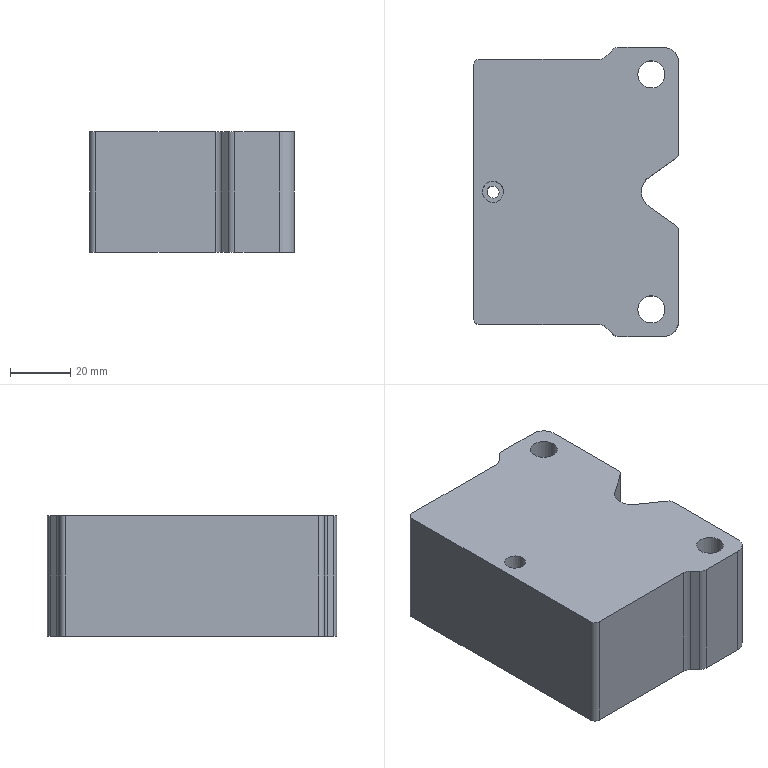Part | NX | features PS-41 2 | 1 solid | 33 faces | box 68 x 96 x 40 mm | volume 229796 mm3 | cylinder 17 | plane 16 | commonest cylinder face diameters 4 x4 6 x4 9 x2 10 x2 14.5 x2 4.001 x1
STEP:
#1=CARTESIAN_POINT('',(4197.993,-814.122,900.716));
#2=VERTEX_POINT('',#1);
#3=CARTESIAN_POINT('',(4158.236,-814.122,900.716));
#4=VERTEX_POINT('',#3);
#5=CARTESIAN_POINT('',(4222.236,-814.122,900.716));
#6=DIRECTION('',(-1.,0.,0.));
#7=VECTOR('',#6,1000.);
#8=LINE('',#5,#7);
#9=EDGE_CURVE('',#2,#4,#8,.T.);
#10=ORIENTED_EDGE('',*,*,#9,.F.);
#11=CARTESIAN_POINT('',(4197.993,-814.122,860.716));
#12=VERTEX_POINT('',#11);
#13=CARTESIAN_POINT('',(4197.993,-814.122,860.716));
#14=DIRECTION('',(0.,0.,-1.));
#15=VECTOR('',#14,1000.);
#16=LINE('',#13,#15);
#17=EDGE_CURVE('',#2,#12,#16,.T.);
#18=ORIENTED_EDGE('',*,*,#17,.T.);
#19=CARTESIAN_POINT('',(4158.236,-814.122,860.716));
#20=VERTEX_POINT('',#19);
#21=CARTESIAN_POINT('',(4222.236,-814.122,860.716));
#22=DIRECTION('',(-1.,0.,0.));
#23=VECTOR('',#22,1000.);
#24=LINE('',#21,#23);
#25=EDGE_CURVE('',#12,#20,#24,.T.);
#26=ORIENTED_EDGE('',*,*,#25,.T.);
#27=CARTESIAN_POINT('',(4158.236,-814.122,860.716));
#28=DIRECTION('',(0.,0.,-1.));
#29=VECTOR('',#28,1000.);
#30=LINE('',#27,#29);
#31=EDGE_CURVE('',#20,#4,#30,.F.);
#32=ORIENTED_EDGE('',*,*,#31,.T.);
#33=EDGE_LOOP('',(#10,#18,#26,#32));
#34=FACE_BOUND('',#33,.T.);
#35=CARTESIAN_POINT('',(4201.082,-814.122,860.716));
#36=DIRECTION('',(0.,1.,0.));
#37=DIRECTION('',(0.,0.,1.));
#38=AXIS2_PLACEMENT_3D('',#35,#36,#37);
#39=PLANE('',#38);
#40=ADVANCED_FACE('',(#34),#39,.T.);
#41=CARTESIAN_POINT('',(4219.736,-819.122,900.716));
#42=VERTEX_POINT('',#41);
#43=CARTESIAN_POINT('',(4215.236,-819.122,900.716));
#44=DIRECTION('',(0.,0.,1.));
#45=DIRECTION('',(1.,0.,0.));
#46=AXIS2_PLACEMENT_3D('',#43,#44,#45);
#47=CIRCLE('',#46,4.5);
#48=EDGE_CURVE('',#42,#42,#47,.T.);
#49=ORIENTED_EDGE('',*,*,#48,.F.);
#50=EDGE_LOOP('',(#49));
#51=FACE_BOUND('',#50,.T.);
#52=CARTESIAN_POINT('',(4219.736,-897.122,900.716));
#53=VERTEX_POINT('',#52);
#54=CARTESIAN_POINT('',(4215.236,-897.122,900.716));
#55=DIRECTION('',(0.,0.,1.));
#56=DIRECTION('',(1.,0.,0.));
#57=AXIS2_PLACEMENT_3D('',#54,#55,#56);
#58=CIRCLE('',#57,4.5);
#59=EDGE_CURVE('',#53,#53,#58,.T.);
#60=ORIENTED_EDGE('',*,*,#59,.F.);
#61=EDGE_LOOP('',(#60));
#62=FACE_BOUND('',#61,.T.);
#63=CARTESIAN_POINT('',(4166.199,-858.122,900.716));
#64=VERTEX_POINT('',#63);
#65=CARTESIAN_POINT('',(4162.699,-858.122,900.716));
#66=DIRECTION('',(0.,0.,1.));
#67=DIRECTION('',(1.,0.,0.));
#68=AXIS2_PLACEMENT_3D('',#65,#66,#67);
#69=CIRCLE('',#68,3.5);
#70=EDGE_CURVE('',#64,#64,#69,.F.);
#71=ORIENTED_EDGE('',*,*,#70,.T.);
#72=EDGE_LOOP('',(#71));
#73=FACE_BOUND('',#72,.T.);
#74=CARTESIAN_POINT('',(4204.479,-906.122,900.716));
#75=VERTEX_POINT('',#74);
#76=CARTESIAN_POINT('',(4219.236,-906.122,900.716));
#77=VERTEX_POINT('',#76);
#78=CARTESIAN_POINT('',(4222.236,-906.122,900.716));
#79=DIRECTION('',(1.,0.,0.));
#80=VECTOR('',#79,1000.);
#81=LINE('',#78,#80);
#82=EDGE_CURVE('',#75,#77,#81,.T.);
#83=ORIENTED_EDGE('',*,*,#82,.T.);
#84=CARTESIAN_POINT('',(4224.236,-901.122,900.716));
#85=VERTEX_POINT('',#84);
#86=CARTESIAN_POINT('',(4219.236,-901.122,900.716));
#87=DIRECTION('',(0.,0.,1.));
#88=DIRECTION('',(1.,0.,0.));
#89=AXIS2_PLACEMENT_3D('',#86,#87,#88);
#90=CIRCLE('',#89,5.);
#91=EDGE_CURVE('',#77,#85,#90,.T.);
#92=ORIENTED_EDGE('',*,*,#91,.T.);
#93=CARTESIAN_POINT('',(4224.236,-870.854,900.716));
#94=VERTEX_POINT('',#93);
#95=CARTESIAN_POINT('',(4224.236,-880.935,900.716));
#96=DIRECTION('',(0.,1.,0.));
#97=VECTOR('',#96,1000.);
#98=LINE('',#95,#97);
#99=EDGE_CURVE('',#85,#94,#98,.T.);
#100=ORIENTED_EDGE('',*,*,#99,.T.);
#101=CARTESIAN_POINT('',(4223.377,-869.212,900.716));
#102=VERTEX_POINT('',#101);
#103=CARTESIAN_POINT('',(4222.236,-870.854,900.716));
#104=DIRECTION('',(0.,0.,1.));
#105=DIRECTION('',(1.,0.,0.));
#106=AXIS2_PLACEMENT_3D('',#103,#104,#105);
#107=CIRCLE('',#106,2.);
#108=EDGE_CURVE('',#94,#102,#107,.T.);
#109=ORIENTED_EDGE('',*,*,#108,.T.);
#110=CARTESIAN_POINT('',(4214.506,-863.05,900.716));
#111=VERTEX_POINT('',#110);
#112=CARTESIAN_POINT('',(4228.1,-872.492,900.716));
#113=DIRECTION('',(-0.8213,0.5705,0.));
#114=VECTOR('',#113,1000.);
#115=LINE('',#112,#114);
#116=EDGE_CURVE('',#102,#111,#115,.T.);
#117=ORIENTED_EDGE('',*,*,#116,.T.);
#118=CARTESIAN_POINT('',(4214.506,-853.194,900.716));
#119=VERTEX_POINT('',#118);
#120=CARTESIAN_POINT('',(4217.929,-858.122,900.716));
#121=DIRECTION('',(0.,0.,1.));
#122=DIRECTION('',(1.,0.,0.));
#123=AXIS2_PLACEMENT_3D('',#120,#121,#122);
#124=CIRCLE('',#123,6.);
#125=EDGE_CURVE('',#111,#119,#124,.F.);
#126=ORIENTED_EDGE('',*,*,#125,.T.);
#127=CARTESIAN_POINT('',(4223.377,-847.032,900.716));
#128=VERTEX_POINT('',#127);
#129=CARTESIAN_POINT('',(4206.723,-858.6,900.716));
#130=DIRECTION('',(0.8213,0.5705,0.));
#131=VECTOR('',#130,1000.);
#132=LINE('',#129,#131);
#133=EDGE_CURVE('',#119,#128,#132,.T.);
#134=ORIENTED_EDGE('',*,*,#133,.T.);
#135=CARTESIAN_POINT('',(4224.236,-845.39,900.716));
#136=VERTEX_POINT('',#135);
#137=CARTESIAN_POINT('',(4222.236,-845.39,900.716));
#138=DIRECTION('',(0.,0.,1.));
#139=DIRECTION('',(1.,0.,0.));
#140=AXIS2_PLACEMENT_3D('',#137,#138,#139);
#141=CIRCLE('',#140,2.);
#142=EDGE_CURVE('',#128,#136,#141,.T.);
#143=ORIENTED_EDGE('',*,*,#142,.T.);
#144=CARTESIAN_POINT('',(4224.236,-815.122,900.716));
#145=VERTEX_POINT('',#144);
#146=CARTESIAN_POINT('',(4224.236,-880.935,900.716));
#147=DIRECTION('',(0.,1.,0.));
#148=VECTOR('',#147,1000.);
#149=LINE('',#146,#148);
#150=EDGE_CURVE('',#136,#145,#149,.T.);
#151=ORIENTED_EDGE('',*,*,#150,.T.);
#152=CARTESIAN_POINT('',(4219.236,-810.122,900.716));
#153=VERTEX_POINT('',#152);
#154=CARTESIAN_POINT('',(4219.236,-815.122,900.716));
#155=DIRECTION('',(0.,0.,1.));
#156=DIRECTION('',(1.,0.,0.));
#157=AXIS2_PLACEMENT_3D('',#154,#155,#156);
#158=CIRCLE('',#157,5.);
#159=EDGE_CURVE('',#145,#153,#158,.T.);
#160=ORIENTED_EDGE('',*,*,#159,.T.);
#161=CARTESIAN_POINT('',(4204.479,-810.122,900.716));
#162=VERTEX_POINT('',#161);
#163=CARTESIAN_POINT('',(4222.236,-810.122,900.716));
#164=DIRECTION('',(-1.,0.,0.));
#165=VECTOR('',#164,1000.);
#166=LINE('',#163,#165);
#167=EDGE_CURVE('',#153,#162,#166,.T.);
#168=ORIENTED_EDGE('',*,*,#167,.T.);
#169=CARTESIAN_POINT('',(4202.357,-811.001,900.716));
#170=VERTEX_POINT('',#169);
#171=CARTESIAN_POINT('',(4204.479,-813.122,900.716));
#172=DIRECTION('',(0.,0.,1.));
#173=DIRECTION('',(1.,0.,0.));
#174=AXIS2_PLACEMENT_3D('',#171,#172,#173);
#175=CIRCLE('',#174,3.);
#176=EDGE_CURVE('',#162,#170,#175,.T.);
#177=ORIENTED_EDGE('',*,*,#176,.T.);
#178=CARTESIAN_POINT('',(4200.115,-813.244,900.716));
#179=VERTEX_POINT('',#178);
#180=CARTESIAN_POINT('',(4199.236,-814.122,900.716));
#181=DIRECTION('',(-0.7071,-0.7071,0.));
#182=VECTOR('',#181,1000.);
#183=LINE('',#180,#182);
#184=EDGE_CURVE('',#170,#179,#183,.T.);
#185=ORIENTED_EDGE('',*,*,#184,.T.);
#186=CARTESIAN_POINT('',(4197.993,-811.122,900.716));
#187=DIRECTION('',(0.,0.,1.));
#188=DIRECTION('',(1.,0.,0.));
#189=AXIS2_PLACEMENT_3D('',#186,#187,#188);
#190=CIRCLE('',#189,3.);
#191=EDGE_CURVE('',#179,#2,#190,.F.);
#192=ORIENTED_EDGE('',*,*,#191,.T.);
#193=ORIENTED_EDGE('',*,*,#9,.T.);
#194=CARTESIAN_POINT('',(4156.236,-816.122,900.716));
#195=VERTEX_POINT('',#194);
#196=CARTESIAN_POINT('',(4158.236,-816.122,900.716));
#197=DIRECTION('',(0.,0.,1.));
#198=DIRECTION('',(1.,0.,0.));
#199=AXIS2_PLACEMENT_3D('',#196,#197,#198);
#200=CIRCLE('',#199,2.);
#201=EDGE_CURVE('',#4,#195,#200,.T.);
#202=ORIENTED_EDGE('',*,*,#201,.T.);
#203=CARTESIAN_POINT('',(4156.236,-900.122,900.716));
#204=VERTEX_POINT('',#203);
#205=CARTESIAN_POINT('',(4156.236,-880.935,900.716));
#206=DIRECTION('',(0.,-1.,0.));
#207=VECTOR('',#206,1000.);
#208=LINE('',#205,#207);
#209=EDGE_CURVE('',#195,#204,#208,.T.);
#210=ORIENTED_EDGE('',*,*,#209,.T.);
#211=CARTESIAN_POINT('',(4158.236,-902.122,900.716));
#212=VERTEX_POINT('',#211);
#213=CARTESIAN_POINT('',(4158.236,-900.122,900.716));
#214=DIRECTION('',(0.,0.,1.));
#215=DIRECTION('',(1.,0.,0.));
#216=AXIS2_PLACEMENT_3D('',#213,#214,#215);
#217=CIRCLE('',#216,2.);
#218=EDGE_CURVE('',#204,#212,#217,.T.);
#219=ORIENTED_EDGE('',*,*,#218,.T.);
#220=CARTESIAN_POINT('',(4197.993,-902.122,900.716));
#221=VERTEX_POINT('',#220);
#222=CARTESIAN_POINT('',(4222.236,-902.122,900.716));
#223=DIRECTION('',(1.,0.,0.));
#224=VECTOR('',#223,1000.);
#225=LINE('',#222,#224);
#226=EDGE_CURVE('',#212,#221,#225,.T.);
#227=ORIENTED_EDGE('',*,*,#226,.T.);
#228=CARTESIAN_POINT('',(4200.115,-903.001,900.716));
#229=VERTEX_POINT('',#228);
#230=CARTESIAN_POINT('',(4197.993,-905.122,900.716));
#231=DIRECTION('',(0.,0.,1.));
#232=DIRECTION('',(1.,0.,0.));
#233=AXIS2_PLACEMENT_3D('',#230,#231,#232);
#234=CIRCLE('',#233,3.);
#235=EDGE_CURVE('',#221,#229,#234,.F.);
#236=ORIENTED_EDGE('',*,*,#235,.T.);
#237=CARTESIAN_POINT('',(4202.357,-905.244,900.716));
#238=VERTEX_POINT('',#237);
#239=CARTESIAN_POINT('',(4199.236,-902.122,900.716));
#240=DIRECTION('',(0.7071,-0.7071,0.));
#241=VECTOR('',#240,1000.);
#242=LINE('',#239,#241);
#243=EDGE_CURVE('',#229,#238,#242,.T.);
#244=ORIENTED_EDGE('',*,*,#243,.T.);
#245=CARTESIAN_POINT('',(4204.479,-903.122,900.716));
#246=DIRECTION('',(0.,0.,1.));
#247=DIRECTION('',(1.,0.,0.));
#248=AXIS2_PLACEMENT_3D('',#245,#246,#247);
#249=CIRCLE('',#248,3.);
#250=EDGE_CURVE('',#238,#75,#249,.T.);
#251=ORIENTED_EDGE('',*,*,#250,.T.);
#252=EDGE_LOOP('',(#83,#92,#100,#109,#117,#126,#134,#143,#151,#160,#168,#177,#185,#192,#193,#202,#210,#219,#227,#236,#244,#251));
#253=FACE_BOUND('',#252,.T.);
#254=CARTESIAN_POINT('',(4222.236,-880.935,900.716));
#255=DIRECTION('',(0.,0.,1.));
#256=DIRECTION('',(1.,0.,0.));
#257=AXIS2_PLACEMENT_3D('',#254,#255,#256);
#258=PLANE('',#257);
#259=ADVANCED_FACE('',(#51,#62,#73,#253),#258,.T.);
#260=CARTESIAN_POINT('',(4222.486,-819.122,860.716));
#261=VERTEX_POINT('',#260);
#262=CARTESIAN_POINT('',(4215.236,-819.122,860.716));
#263=DIRECTION('',(0.,0.,1.));
#264=DIRECTION('',(1.,0.,0.));
#265=AXIS2_PLACEMENT_3D('',#262,#263,#264);
#266=CIRCLE('',#265,7.25);
#267=EDGE_CURVE('',#261,#261,#266,.T.);
#268=ORIENTED_EDGE('',*,*,#267,.T.);
#269=EDGE_LOOP('',(#268));
#270=FACE_BOUND('',#269,.T.);
#271=CARTESIAN_POINT('',(4222.486,-897.122,860.716));
#272=VERTEX_POINT('',#271);
#273=CARTESIAN_POINT('',(4215.236,-897.122,860.716));
#274=DIRECTION('',(0.,0.,1.));
#275=DIRECTION('',(1.,0.,0.));
#276=AXIS2_PLACEMENT_3D('',#273,#274,#275);
#277=CIRCLE('',#276,7.25);
#278=EDGE_CURVE('',#272,#272,#277,.T.);
#279=ORIENTED_EDGE('',*,*,#278,.T.);
#280=EDGE_LOOP('',(#279));
#281=FACE_BOUND('',#280,.T.);
#282=CARTESIAN_POINT('',(4164.699,-858.122,860.716));
#283=VERTEX_POINT('',#282);
#284=CARTESIAN_POINT('',(4162.699,-858.122,860.716));
#285=DIRECTION('',(0.,0.,1.));
#286=DIRECTION('',(1.,0.,0.));
#287=AXIS2_PLACEMENT_3D('',#284,#285,#286);
#288=CIRCLE('',#287,2.001);
#289=EDGE_CURVE('',#283,#283,#288,.T.);
#290=ORIENTED_EDGE('',*,*,#289,.T.);
#291=EDGE_LOOP('',(#290));
#292=FACE_BOUND('',#291,.T.);
#293=CARTESIAN_POINT('',(4224.236,-901.122,860.716));
#294=VERTEX_POINT('',#293);
#295=CARTESIAN_POINT('',(4224.236,-870.854,860.716));
#296=VERTEX_POINT('',#295);
#297=CARTESIAN_POINT('',(4224.236,-880.935,860.716));
#298=DIRECTION('',(0.,1.,0.));
#299=VECTOR('',#298,1000.);
#300=LINE('',#297,#299);
#301=EDGE_CURVE('',#294,#296,#300,.T.);
#302=ORIENTED_EDGE('',*,*,#301,.F.);
#303=CARTESIAN_POINT('',(4219.236,-906.122,860.716));
#304=VERTEX_POINT('',#303);
#305=CARTESIAN_POINT('',(4219.236,-901.122,860.716));
#306=DIRECTION('',(0.,0.,1.));
#307=DIRECTION('',(1.,0.,0.));
#308=AXIS2_PLACEMENT_3D('',#305,#306,#307);
#309=CIRCLE('',#308,5.);
#310=EDGE_CURVE('',#294,#304,#309,.F.);
#311=ORIENTED_EDGE('',*,*,#310,.T.);
#312=CARTESIAN_POINT('',(4204.479,-906.122,860.716));
#313=VERTEX_POINT('',#312);
#314=CARTESIAN_POINT('',(4222.236,-906.122,860.716));
#315=DIRECTION('',(1.,0.,0.));
#316=VECTOR('',#315,1000.);
#317=LINE('',#314,#316);
#318=EDGE_CURVE('',#313,#304,#317,.T.);
#319=ORIENTED_EDGE('',*,*,#318,.F.);
#320=CARTESIAN_POINT('',(4202.357,-905.244,860.716));
#321=VERTEX_POINT('',#320);
#322=CARTESIAN_POINT('',(4204.479,-903.122,860.716));
#323=DIRECTION('',(0.,0.,1.));
#324=DIRECTION('',(1.,0.,0.));
#325=AXIS2_PLACEMENT_3D('',#322,#323,#324);
#326=CIRCLE('',#325,3.);
#327=EDGE_CURVE('',#313,#321,#326,.F.);
#328=ORIENTED_EDGE('',*,*,#327,.T.);
#329=CARTESIAN_POINT('',(4200.115,-903.001,860.716));
#330=VERTEX_POINT('',#329);
#331=CARTESIAN_POINT('',(4200.142,-903.028,860.716));
#332=DIRECTION('',(-0.7071,0.7071,0.));
#333=VECTOR('',#332,1000.);
#334=LINE('',#331,#333);
#335=EDGE_CURVE('',#321,#330,#334,.T.);
#336=ORIENTED_EDGE('',*,*,#335,.T.);
#337=CARTESIAN_POINT('',(4197.993,-902.122,860.716));
#338=VERTEX_POINT('',#337);
#339=CARTESIAN_POINT('',(4197.993,-905.122,860.716));
#340=DIRECTION('',(0.,0.,1.));
#341=DIRECTION('',(1.,0.,0.));
#342=AXIS2_PLACEMENT_3D('',#339,#340,#341);
#343=CIRCLE('',#342,3.);
#344=EDGE_CURVE('',#330,#338,#343,.T.);
#345=ORIENTED_EDGE('',*,*,#344,.T.);
#346=CARTESIAN_POINT('',(4158.236,-902.122,860.716));
#347=VERTEX_POINT('',#346);
#348=CARTESIAN_POINT('',(4222.236,-902.122,860.716));
#349=DIRECTION('',(1.,0.,0.));
#350=VECTOR('',#349,1000.);
#351=LINE('',#348,#350);
#352=EDGE_CURVE('',#347,#338,#351,.T.);
#353=ORIENTED_EDGE('',*,*,#352,.F.);
#354=CARTESIAN_POINT('',(4156.236,-900.122,860.716));
#355=VERTEX_POINT('',#354);
#356=CARTESIAN_POINT('',(4158.236,-900.122,860.716));
#357=DIRECTION('',(0.,0.,1.));
#358=DIRECTION('',(1.,0.,0.));
#359=AXIS2_PLACEMENT_3D('',#356,#357,#358);
#360=CIRCLE('',#359,2.);
#361=EDGE_CURVE('',#347,#355,#360,.F.);
#362=ORIENTED_EDGE('',*,*,#361,.T.);
#363=CARTESIAN_POINT('',(4156.236,-816.122,860.716));
#364=VERTEX_POINT('',#363);
#365=CARTESIAN_POINT('',(4156.236,-799.122,860.716));
#366=DIRECTION('',(0.,-1.,0.));
#367=VECTOR('',#366,1000.);
#368=LINE('',#365,#367);
#369=EDGE_CURVE('',#364,#355,#368,.T.);
#370=ORIENTED_EDGE('',*,*,#369,.F.);
#371=CARTESIAN_POINT('',(4158.236,-816.122,860.716));
#372=DIRECTION('',(0.,0.,1.));
#373=DIRECTION('',(1.,0.,0.));
#374=AXIS2_PLACEMENT_3D('',#371,#372,#373);
#375=CIRCLE('',#374,2.);
#376=EDGE_CURVE('',#364,#20,#375,.F.);
#377=ORIENTED_EDGE('',*,*,#376,.T.);
#378=ORIENTED_EDGE('',*,*,#25,.F.);
#379=CARTESIAN_POINT('',(4200.115,-813.244,860.716));
#380=VERTEX_POINT('',#379);
#381=CARTESIAN_POINT('',(4197.993,-811.122,860.716));
#382=DIRECTION('',(0.,0.,1.));
#383=DIRECTION('',(1.,0.,0.));
#384=AXIS2_PLACEMENT_3D('',#381,#382,#383);
#385=CIRCLE('',#384,3.);
#386=EDGE_CURVE('',#12,#380,#385,.T.);
#387=ORIENTED_EDGE('',*,*,#386,.T.);
#388=CARTESIAN_POINT('',(4202.357,-811.001,860.716));
#389=VERTEX_POINT('',#388);
#390=CARTESIAN_POINT('',(4177.33,-836.028,860.716));
#391=DIRECTION('',(0.7071,0.7071,0.));
#392=VECTOR('',#391,1000.);
#393=LINE('',#390,#392);
#394=EDGE_CURVE('',#380,#389,#393,.T.);
#395=ORIENTED_EDGE('',*,*,#394,.T.);
#396=CARTESIAN_POINT('',(4204.479,-810.122,860.716));
#397=VERTEX_POINT('',#396);
#398=CARTESIAN_POINT('',(4204.479,-813.122,860.716));
#399=DIRECTION('',(0.,0.,1.));
#400=DIRECTION('',(1.,0.,0.));
#401=AXIS2_PLACEMENT_3D('',#398,#399,#400);
#402=CIRCLE('',#401,3.);
#403=EDGE_CURVE('',#389,#397,#402,.F.);
#404=ORIENTED_EDGE('',*,*,#403,.T.);
#405=CARTESIAN_POINT('',(4219.236,-810.122,860.716));
#406=VERTEX_POINT('',#405);
#407=CARTESIAN_POINT('',(4222.236,-810.122,860.716));
#408=DIRECTION('',(-1.,0.,0.));
#409=VECTOR('',#408,1000.);
#410=LINE('',#407,#409);
#411=EDGE_CURVE('',#406,#397,#410,.T.);
#412=ORIENTED_EDGE('',*,*,#411,.F.);
#413=CARTESIAN_POINT('',(4224.236,-815.122,860.716));
#414=VERTEX_POINT('',#413);
#415=CARTESIAN_POINT('',(4219.236,-815.122,860.716));
#416=DIRECTION('',(0.,0.,1.));
#417=DIRECTION('',(1.,0.,0.));
#418=AXIS2_PLACEMENT_3D('',#415,#416,#417);
#419=CIRCLE('',#418,5.);
#420=EDGE_CURVE('',#406,#414,#419,.F.);
#421=ORIENTED_EDGE('',*,*,#420,.T.);
#422=CARTESIAN_POINT('',(4224.236,-845.39,860.716));
#423=VERTEX_POINT('',#422);
#424=CARTESIAN_POINT('',(4224.236,-845.39,860.716));
#425=DIRECTION('',(0.,1.,0.));
#426=VECTOR('',#425,1000.);
#427=LINE('',#424,#426);
#428=EDGE_CURVE('',#423,#414,#427,.T.);
#429=ORIENTED_EDGE('',*,*,#428,.F.);
#430=CARTESIAN_POINT('',(4223.377,-847.032,860.716));
#431=VERTEX_POINT('',#430);
#432=CARTESIAN_POINT('',(4222.236,-845.39,860.716));
#433=DIRECTION('',(0.,0.,1.));
#434=DIRECTION('',(1.,0.,0.));
#435=AXIS2_PLACEMENT_3D('',#432,#433,#434);
#436=CIRCLE('',#435,2.);
#437=EDGE_CURVE('',#431,#423,#436,.T.);
#438=ORIENTED_EDGE('',*,*,#437,.F.);
#439=CARTESIAN_POINT('',(4214.506,-853.194,860.716));
#440=VERTEX_POINT('',#439);
#441=CARTESIAN_POINT('',(4214.506,-853.194,860.716));
#442=DIRECTION('',(0.8213,0.5705,0.));
#443=VECTOR('',#442,1000.);
#444=LINE('',#441,#443);
#445=EDGE_CURVE('',#440,#431,#444,.T.);
#446=ORIENTED_EDGE('',*,*,#445,.F.);
#447=CARTESIAN_POINT('',(4214.506,-863.05,860.716));
#448=VERTEX_POINT('',#447);
#449=CARTESIAN_POINT('',(4217.929,-858.122,860.716));
#450=DIRECTION('',(0.,0.,-1.));
#451=DIRECTION('',(1.,0.,0.));
#452=AXIS2_PLACEMENT_3D('',#449,#450,#451);
#453=CIRCLE('',#452,6.);
#454=EDGE_CURVE('',#448,#440,#453,.T.);
#455=ORIENTED_EDGE('',*,*,#454,.F.);
#456=CARTESIAN_POINT('',(4223.377,-869.212,860.716));
#457=VERTEX_POINT('',#456);
#458=CARTESIAN_POINT('',(4223.377,-869.212,860.716));
#459=DIRECTION('',(-0.8213,0.5705,0.));
#460=VECTOR('',#459,1000.);
#461=LINE('',#458,#460);
#462=EDGE_CURVE('',#457,#448,#461,.T.);
#463=ORIENTED_EDGE('',*,*,#462,.F.);
#464=CARTESIAN_POINT('',(4222.236,-870.854,860.716));
#465=DIRECTION('',(0.,0.,1.));
#466=DIRECTION('',(1.,0.,0.));
#467=AXIS2_PLACEMENT_3D('',#464,#465,#466);
#468=CIRCLE('',#467,2.);
#469=EDGE_CURVE('',#296,#457,#468,.T.);
#470=ORIENTED_EDGE('',*,*,#469,.F.);
#471=EDGE_LOOP('',(#302,#311,#319,#328,#336,#345,#353,#362,#370,#377,#378,#387,#395,#404,#412,#421,#429,#438,#446,#455,#463,#470));
#472=FACE_BOUND('',#471,.T.);
#473=CARTESIAN_POINT('',(4222.236,-880.935,860.716));
#474=DIRECTION('',(0.,0.,1.));
#475=DIRECTION('',(1.,0.,0.));
#476=AXIS2_PLACEMENT_3D('',#473,#474,#475);
#477=PLANE('',#476);
#478=ADVANCED_FACE('',(#270,#281,#292,#472),#477,.F.);
#479=ORIENTED_EDGE('',*,*,#352,.T.);
#480=CARTESIAN_POINT('',(4197.993,-902.122,860.716));
#481=DIRECTION('',(0.,0.,1.));
#482=VECTOR('',#481,1000.);
#483=LINE('',#480,#482);
#484=EDGE_CURVE('',#338,#221,#483,.T.);
#485=ORIENTED_EDGE('',*,*,#484,.T.);
#486=ORIENTED_EDGE('',*,*,#226,.F.);
#487=CARTESIAN_POINT('',(4158.236,-902.122,860.716));
#488=DIRECTION('',(0.,0.,1.));
#489=VECTOR('',#488,1000.);
#490=LINE('',#487,#489);
#491=EDGE_CURVE('',#212,#347,#490,.F.);
#492=ORIENTED_EDGE('',*,*,#491,.T.);
#493=EDGE_LOOP('',(#479,#485,#486,#492));
#494=FACE_BOUND('',#493,.T.);
#495=CARTESIAN_POINT('',(4184.236,-902.122,860.716));
#496=DIRECTION('',(0.,-1.,0.));
#497=DIRECTION('',(0.,0.,-1.));
#498=AXIS2_PLACEMENT_3D('',#495,#496,#497);
#499=PLANE('',#498);
#500=ADVANCED_FACE('',(#494),#499,.T.);
#501=CARTESIAN_POINT('',(4161.284,-856.708,877.716));
#502=VERTEX_POINT('',#501);
#503=CARTESIAN_POINT('',(4162.699,-858.122,877.716));
#504=DIRECTION('',(0.,0.,-1.));
#505=DIRECTION('',(-0.7071,0.7071,0.));
#506=AXIS2_PLACEMENT_3D('',#503,#504,#505);
#507=CIRCLE('',#506,2.001);
#508=EDGE_CURVE('',#502,#502,#507,.T.);
#509=ORIENTED_EDGE('',*,*,#508,.T.);
#510=EDGE_LOOP('',(#509));
#511=FACE_BOUND('',#510,.T.);
#512=CARTESIAN_POINT('',(4165.174,-860.597,877.716));
#513=VERTEX_POINT('',#512);
#514=CARTESIAN_POINT('',(4162.699,-858.122,877.716));
#515=DIRECTION('',(0.,0.,1.));
#516=DIRECTION('',(0.7071,-0.7071,0.));
#517=AXIS2_PLACEMENT_3D('',#514,#515,#516);
#518=CIRCLE('',#517,3.5);
#519=EDGE_CURVE('',#513,#513,#518,.F.);
#520=ORIENTED_EDGE('',*,*,#519,.F.);
#521=EDGE_LOOP('',(#520));
#522=FACE_BOUND('',#521,.T.);
#523=CARTESIAN_POINT('',(4162.699,-858.122,877.716));
#524=DIRECTION('',(0.,0.,-1.));
#525=DIRECTION('',(-0.7071,0.7071,0.));
#526=AXIS2_PLACEMENT_3D('',#523,#524,#525);
#527=PLANE('',#526);
#528=ADVANCED_FACE('',(#511,#522),#527,.F.);
#529=ORIENTED_EDGE('',*,*,#508,.F.);
#530=EDGE_LOOP('',(#529));
#531=FACE_BOUND('',#530,.T.);
#532=ORIENTED_EDGE('',*,*,#289,.F.);
#533=EDGE_LOOP('',(#532));
#534=FACE_BOUND('',#533,.T.);
#535=CARTESIAN_POINT('',(4162.699,-858.122,887.716));
#536=DIRECTION('',(0.,0.,-1.));
#537=DIRECTION('',(0.7071,-0.7071,0.));
#538=AXIS2_PLACEMENT_3D('',#535,#536,#537);
#539=CYLINDRICAL_SURFACE('',#538,2.001);
#540=ADVANCED_FACE('',(#531,#534),#539,.F.);
#541=ORIENTED_EDGE('',*,*,#519,.T.);
#542=EDGE_LOOP('',(#541));
#543=FACE_BOUND('',#542,.T.);
#544=ORIENTED_EDGE('',*,*,#70,.F.);
#545=EDGE_LOOP('',(#544));
#546=FACE_BOUND('',#545,.T.);
#547=CARTESIAN_POINT('',(4162.699,-858.122,887.716));
#548=DIRECTION('',(0.,0.,-1.));
#549=DIRECTION('',(0.7071,-0.7071,0.));
#550=AXIS2_PLACEMENT_3D('',#547,#548,#549);
#551=CYLINDRICAL_SURFACE('',#550,3.5);
#552=ADVANCED_FACE('',(#543,#546),#551,.F.);
#553=ORIENTED_EDGE('',*,*,#369,.T.);
#554=CARTESIAN_POINT('',(4156.236,-900.122,860.716));
#555=DIRECTION('',(0.,0.,1.));
#556=VECTOR('',#555,1000.);
#557=LINE('',#554,#556);
#558=EDGE_CURVE('',#355,#204,#557,.T.);
#559=ORIENTED_EDGE('',*,*,#558,.T.);
#560=ORIENTED_EDGE('',*,*,#209,.F.);
#561=CARTESIAN_POINT('',(4156.236,-816.122,860.716));
#562=DIRECTION('',(0.,0.,-1.));
#563=VECTOR('',#562,1000.);
#564=LINE('',#561,#563);
#565=EDGE_CURVE('',#195,#364,#564,.T.);
#566=ORIENTED_EDGE('',*,*,#565,.T.);
#567=EDGE_LOOP('',(#553,#559,#560,#566));
#568=FACE_BOUND('',#567,.T.);
#569=CARTESIAN_POINT('',(4156.236,-799.122,860.716));
#570=DIRECTION('',(-1.,0.,0.));
#571=DIRECTION('',(0.,-1.,0.));
#572=AXIS2_PLACEMENT_3D('',#569,#570,#571);
#573=PLANE('',#572);
#574=ADVANCED_FACE('',(#568),#573,.T.);
#575=ORIENTED_EDGE('',*,*,#361,.F.);
#576=ORIENTED_EDGE('',*,*,#491,.F.);
#577=ORIENTED_EDGE('',*,*,#218,.F.);
#578=ORIENTED_EDGE('',*,*,#558,.F.);
#579=EDGE_LOOP('',(#575,#576,#577,#578));
#580=FACE_BOUND('',#579,.T.);
#581=CARTESIAN_POINT('',(4158.236,-900.122,860.716));
#582=DIRECTION('',(0.,0.,1.));
#583=DIRECTION('',(1.,0.,0.));
#584=AXIS2_PLACEMENT_3D('',#581,#582,#583);
#585=CYLINDRICAL_SURFACE('',#584,2.);
#586=ADVANCED_FACE('',(#580),#585,.T.);
#587=ORIENTED_EDGE('',*,*,#201,.F.);
#588=ORIENTED_EDGE('',*,*,#31,.F.);
#589=ORIENTED_EDGE('',*,*,#376,.F.);
#590=ORIENTED_EDGE('',*,*,#565,.F.);
#591=EDGE_LOOP('',(#587,#588,#589,#590));
#592=FACE_BOUND('',#591,.T.);
#593=CARTESIAN_POINT('',(4158.236,-816.122,860.716));
#594=DIRECTION('',(0.,0.,-1.));
#595=DIRECTION('',(-1.,0.,0.));
#596=AXIS2_PLACEMENT_3D('',#593,#594,#595);
#597=CYLINDRICAL_SURFACE('',#596,2.);
#598=ADVANCED_FACE('',(#592),#597,.T.);
#599=ORIENTED_EDGE('',*,*,#108,.F.);
#600=CARTESIAN_POINT('',(4224.236,-870.854,860.716));
#601=DIRECTION('',(0.,0.,1.));
#602=VECTOR('',#601,1000.);
#603=LINE('',#600,#602);
#604=EDGE_CURVE('',#296,#94,#603,.T.);
#605=ORIENTED_EDGE('',*,*,#604,.F.);
#606=ORIENTED_EDGE('',*,*,#469,.T.);
#607=CARTESIAN_POINT('',(4223.377,-869.212,860.716));
#608=DIRECTION('',(0.,0.,1.));
#609=VECTOR('',#608,1000.);
#610=LINE('',#607,#609);
#611=EDGE_CURVE('',#457,#102,#610,.T.);
#612=ORIENTED_EDGE('',*,*,#611,.T.);
#613=EDGE_LOOP('',(#599,#605,#606,#612));
#614=FACE_BOUND('',#613,.T.);
#615=CARTESIAN_POINT('',(4222.236,-870.854,860.716));
#616=DIRECTION('',(0.,0.,1.));
#617=DIRECTION('',(1.,0.,0.));
#618=AXIS2_PLACEMENT_3D('',#615,#616,#617);
#619=CYLINDRICAL_SURFACE('',#618,2.);
#620=ADVANCED_FACE('',(#614),#619,.T.);
#621=ORIENTED_EDGE('',*,*,#116,.F.);
#622=ORIENTED_EDGE('',*,*,#611,.F.);
#623=ORIENTED_EDGE('',*,*,#462,.T.);
#624=CARTESIAN_POINT('',(4214.506,-863.05,860.716));
#625=DIRECTION('',(0.,0.,1.));
#626=VECTOR('',#625,1000.);
#627=LINE('',#624,#626);
#628=EDGE_CURVE('',#448,#111,#627,.T.);
#629=ORIENTED_EDGE('',*,*,#628,.T.);
#630=EDGE_LOOP('',(#621,#622,#623,#629));
#631=FACE_BOUND('',#630,.T.);
#632=CARTESIAN_POINT('',(4223.377,-869.212,860.716));
#633=DIRECTION('',(0.5705,0.8213,0.));
#634=DIRECTION('',(-0.8213,0.5705,0.));
#635=AXIS2_PLACEMENT_3D('',#632,#633,#634);
#636=PLANE('',#635);
#637=ADVANCED_FACE('',(#631),#636,.T.);
#638=ORIENTED_EDGE('',*,*,#125,.F.);
#639=ORIENTED_EDGE('',*,*,#628,.F.);
#640=ORIENTED_EDGE('',*,*,#454,.T.);
#641=CARTESIAN_POINT('',(4214.506,-853.194,860.716));
#642=DIRECTION('',(0.,0.,1.));
#643=VECTOR('',#642,1000.);
#644=LINE('',#641,#643);
#645=EDGE_CURVE('',#440,#119,#644,.T.);
#646=ORIENTED_EDGE('',*,*,#645,.T.);
#647=EDGE_LOOP('',(#638,#639,#640,#646));
#648=FACE_BOUND('',#647,.T.);
#649=CARTESIAN_POINT('',(4217.929,-858.122,860.716));
#650=DIRECTION('',(0.,0.,1.));
#651=DIRECTION('',(1.,0.,0.));
#652=AXIS2_PLACEMENT_3D('',#649,#650,#651);
#653=CYLINDRICAL_SURFACE('',#652,6.);
#654=ADVANCED_FACE('',(#648),#653,.F.);
#655=ORIENTED_EDGE('',*,*,#133,.F.);
#656=ORIENTED_EDGE('',*,*,#645,.F.);
#657=ORIENTED_EDGE('',*,*,#445,.T.);
#658=CARTESIAN_POINT('',(4223.377,-847.032,860.716));
#659=DIRECTION('',(0.,0.,1.));
#660=VECTOR('',#659,1000.);
#661=LINE('',#658,#660);
#662=EDGE_CURVE('',#431,#128,#661,.T.);
#663=ORIENTED_EDGE('',*,*,#662,.T.);
#664=EDGE_LOOP('',(#655,#656,#657,#663));
#665=FACE_BOUND('',#664,.T.);
#666=CARTESIAN_POINT('',(4214.506,-853.194,860.716));
#667=DIRECTION('',(0.5705,-0.8213,0.));
#668=DIRECTION('',(0.8213,0.5705,0.));
#669=AXIS2_PLACEMENT_3D('',#666,#667,#668);
#670=PLANE('',#669);
#671=ADVANCED_FACE('',(#665),#670,.T.);
#672=ORIENTED_EDGE('',*,*,#142,.F.);
#673=ORIENTED_EDGE('',*,*,#662,.F.);
#674=ORIENTED_EDGE('',*,*,#437,.T.);
#675=CARTESIAN_POINT('',(4224.236,-845.39,860.716));
#676=DIRECTION('',(0.,0.,1.));
#677=VECTOR('',#676,1000.);
#678=LINE('',#675,#677);
#679=EDGE_CURVE('',#423,#136,#678,.T.);
#680=ORIENTED_EDGE('',*,*,#679,.T.);
#681=EDGE_LOOP('',(#672,#673,#674,#680));
#682=FACE_BOUND('',#681,.T.);
#683=CARTESIAN_POINT('',(4222.236,-845.39,860.716));
#684=DIRECTION('',(0.,0.,1.));
#685=DIRECTION('',(1.,0.,0.));
#686=AXIS2_PLACEMENT_3D('',#683,#684,#685);
#687=CYLINDRICAL_SURFACE('',#686,2.);
#688=ADVANCED_FACE('',(#682),#687,.T.);
#689=ORIENTED_EDGE('',*,*,#428,.T.);
#690=CARTESIAN_POINT('',(4224.236,-815.122,860.716));
#691=DIRECTION('',(0.,0.,1.));
#692=VECTOR('',#691,1000.);
#693=LINE('',#690,#692);
#694=EDGE_CURVE('',#414,#145,#693,.T.);
#695=ORIENTED_EDGE('',*,*,#694,.T.);
#696=ORIENTED_EDGE('',*,*,#150,.F.);
#697=ORIENTED_EDGE('',*,*,#679,.F.);
#698=EDGE_LOOP('',(#689,#695,#696,#697));
#699=FACE_BOUND('',#698,.T.);
#700=CARTESIAN_POINT('',(4224.236,-845.39,860.716));
#701=DIRECTION('',(1.,0.,0.));
#702=DIRECTION('',(0.,1.,0.));
#703=AXIS2_PLACEMENT_3D('',#700,#701,#702);
#704=PLANE('',#703);
#705=ADVANCED_FACE('',(#699),#704,.T.);
#706=ORIENTED_EDGE('',*,*,#99,.F.);
#707=CARTESIAN_POINT('',(4224.236,-901.122,860.716));
#708=DIRECTION('',(0.,0.,1.));
#709=VECTOR('',#708,1000.);
#710=LINE('',#707,#709);
#711=EDGE_CURVE('',#85,#294,#710,.F.);
#712=ORIENTED_EDGE('',*,*,#711,.T.);
#713=ORIENTED_EDGE('',*,*,#301,.T.);
#714=ORIENTED_EDGE('',*,*,#604,.T.);
#715=EDGE_LOOP('',(#706,#712,#713,#714));
#716=FACE_BOUND('',#715,.T.);
#717=CARTESIAN_POINT('',(4224.236,-880.935,860.716));
#718=DIRECTION('',(1.,0.,0.));
#719=DIRECTION('',(0.,1.,0.));
#720=AXIS2_PLACEMENT_3D('',#717,#718,#719);
#721=PLANE('',#720);
#722=ADVANCED_FACE('',(#716),#721,.T.);
#723=ORIENTED_EDGE('',*,*,#318,.T.);
#724=CARTESIAN_POINT('',(4219.236,-906.122,860.716));
#725=DIRECTION('',(0.,0.,1.));
#726=VECTOR('',#725,1000.);
#727=LINE('',#724,#726);
#728=EDGE_CURVE('',#304,#77,#727,.T.);
#729=ORIENTED_EDGE('',*,*,#728,.T.);
#730=ORIENTED_EDGE('',*,*,#82,.F.);
#731=CARTESIAN_POINT('',(4204.479,-906.122,860.716));
#732=DIRECTION('',(0.,0.,-1.));
#733=VECTOR('',#732,1000.);
#734=LINE('',#731,#733);
#735=EDGE_CURVE('',#75,#313,#734,.T.);
#736=ORIENTED_EDGE('',*,*,#735,.T.);
#737=EDGE_LOOP('',(#723,#729,#730,#736));
#738=FACE_BOUND('',#737,.T.);
#739=CARTESIAN_POINT('',(4184.236,-906.122,860.716));
#740=DIRECTION('',(0.,-1.,0.));
#741=DIRECTION('',(0.,0.,-1.));
#742=AXIS2_PLACEMENT_3D('',#739,#740,#741);
#743=PLANE('',#742);
#744=ADVANCED_FACE('',(#738),#743,.T.);
#745=ORIENTED_EDGE('',*,*,#167,.F.);
#746=CARTESIAN_POINT('',(4219.236,-810.122,860.716));
#747=DIRECTION('',(0.,0.,1.));
#748=VECTOR('',#747,1000.);
#749=LINE('',#746,#748);
#750=EDGE_CURVE('',#153,#406,#749,.F.);
#751=ORIENTED_EDGE('',*,*,#750,.T.);
#752=ORIENTED_EDGE('',*,*,#411,.T.);
#753=CARTESIAN_POINT('',(4204.479,-810.122,900.716));
#754=DIRECTION('',(0.,0.,1.));
#755=VECTOR('',#754,1000.);
#756=LINE('',#753,#755);
#757=EDGE_CURVE('',#397,#162,#756,.T.);
#758=ORIENTED_EDGE('',*,*,#757,.T.);
#759=EDGE_LOOP('',(#745,#751,#752,#758));
#760=FACE_BOUND('',#759,.T.);
#761=CARTESIAN_POINT('',(4201.082,-810.122,860.716));
#762=DIRECTION('',(0.,1.,0.));
#763=DIRECTION('',(0.,0.,1.));
#764=AXIS2_PLACEMENT_3D('',#761,#762,#763);
#765=PLANE('',#764);
#766=ADVANCED_FACE('',(#760),#765,.T.);
#767=ORIENTED_EDGE('',*,*,#335,.F.);
#768=CARTESIAN_POINT('',(4202.357,-905.244,900.716));
#769=DIRECTION('',(0.,0.,-1.));
#770=VECTOR('',#769,1000.);
#771=LINE('',#768,#770);
#772=EDGE_CURVE('',#321,#238,#771,.F.);
#773=ORIENTED_EDGE('',*,*,#772,.T.);
#774=ORIENTED_EDGE('',*,*,#243,.F.);
#775=CARTESIAN_POINT('',(4200.115,-903.001,860.716));
#776=DIRECTION('',(0.,0.,1.));
#777=VECTOR('',#776,1000.);
#778=LINE('',#775,#777);
#779=EDGE_CURVE('',#229,#330,#778,.F.);
#780=ORIENTED_EDGE('',*,*,#779,.T.);
#781=EDGE_LOOP('',(#767,#773,#774,#780));
#782=FACE_BOUND('',#781,.T.);
#783=CARTESIAN_POINT('',(4199.236,-902.122,860.716));
#784=DIRECTION('',(0.7071,0.7071,0.));
#785=DIRECTION('',(0.,0.,1.));
#786=AXIS2_PLACEMENT_3D('',#783,#784,#785);
#787=PLANE('',#786);
#788=ADVANCED_FACE('',(#782),#787,.F.);
#789=ORIENTED_EDGE('',*,*,#184,.F.);
#790=CARTESIAN_POINT('',(4202.357,-811.001,860.716));
#791=DIRECTION('',(0.,0.,1.));
#792=VECTOR('',#791,1000.);
#793=LINE('',#790,#792);
#794=EDGE_CURVE('',#170,#389,#793,.F.);
#795=ORIENTED_EDGE('',*,*,#794,.T.);
#796=ORIENTED_EDGE('',*,*,#394,.F.);
#797=CARTESIAN_POINT('',(4200.115,-813.244,860.716));
#798=DIRECTION('',(0.,0.,-1.));
#799=VECTOR('',#798,1000.);
#800=LINE('',#797,#799);
#801=EDGE_CURVE('',#380,#179,#800,.F.);
#802=ORIENTED_EDGE('',*,*,#801,.T.);
#803=EDGE_LOOP('',(#789,#795,#796,#802));
#804=FACE_BOUND('',#803,.T.);
#805=CARTESIAN_POINT('',(4199.236,-814.122,860.716));
#806=DIRECTION('',(0.7071,-0.7071,0.));
#807=DIRECTION('',(0.,0.,-1.));
#808=AXIS2_PLACEMENT_3D('',#805,#806,#807);
#809=PLANE('',#808);
#810=ADVANCED_FACE('',(#804),#809,.F.);
#811=ORIENTED_EDGE('',*,*,#250,.F.);
#812=ORIENTED_EDGE('',*,*,#772,.F.);
#813=ORIENTED_EDGE('',*,*,#327,.F.);
#814=ORIENTED_EDGE('',*,*,#735,.F.);
#815=EDGE_LOOP('',(#811,#812,#813,#814));
#816=FACE_BOUND('',#815,.T.);
#817=CARTESIAN_POINT('',(4204.479,-903.122,860.716));
#818=DIRECTION('',(0.,0.,1.));
#819=DIRECTION('',(1.,0.,0.));
#820=AXIS2_PLACEMENT_3D('',#817,#818,#819);
#821=CYLINDRICAL_SURFACE('',#820,3.);
#822=ADVANCED_FACE('',(#816),#821,.T.);
#823=ORIENTED_EDGE('',*,*,#344,.F.);
#824=ORIENTED_EDGE('',*,*,#779,.F.);
#825=ORIENTED_EDGE('',*,*,#235,.F.);
#826=ORIENTED_EDGE('',*,*,#484,.F.);
#827=EDGE_LOOP('',(#823,#824,#825,#826));
#828=FACE_BOUND('',#827,.T.);
#829=CARTESIAN_POINT('',(4197.993,-905.122,860.716));
#830=DIRECTION('',(0.,0.,1.));
#831=DIRECTION('',(1.,0.,0.));
#832=AXIS2_PLACEMENT_3D('',#829,#830,#831);
#833=CYLINDRICAL_SURFACE('',#832,3.);
#834=ADVANCED_FACE('',(#828),#833,.F.);
#835=ORIENTED_EDGE('',*,*,#403,.F.);
#836=ORIENTED_EDGE('',*,*,#794,.F.);
#837=ORIENTED_EDGE('',*,*,#176,.F.);
#838=ORIENTED_EDGE('',*,*,#757,.F.);
#839=EDGE_LOOP('',(#835,#836,#837,#838));
#840=FACE_BOUND('',#839,.T.);
#841=CARTESIAN_POINT('',(4204.479,-813.122,860.716));
#842=DIRECTION('',(0.,0.,-1.));
#843=DIRECTION('',(-1.,0.,0.));
#844=AXIS2_PLACEMENT_3D('',#841,#842,#843);
#845=CYLINDRICAL_SURFACE('',#844,3.);
#846=ADVANCED_FACE('',(#840),#845,.T.);
#847=ORIENTED_EDGE('',*,*,#191,.F.);
#848=ORIENTED_EDGE('',*,*,#801,.F.);
#849=ORIENTED_EDGE('',*,*,#386,.F.);
#850=ORIENTED_EDGE('',*,*,#17,.F.);
#851=EDGE_LOOP('',(#847,#848,#849,#850));
#852=FACE_BOUND('',#851,.T.);
#853=CARTESIAN_POINT('',(4197.993,-811.122,860.716));
#854=DIRECTION('',(0.,0.,-1.));
#855=DIRECTION('',(-1.,0.,0.));
#856=AXIS2_PLACEMENT_3D('',#853,#854,#855);
#857=CYLINDRICAL_SURFACE('',#856,3.);
#858=ADVANCED_FACE('',(#852),#857,.F.);
#859=ORIENTED_EDGE('',*,*,#310,.F.);
#860=ORIENTED_EDGE('',*,*,#711,.F.);
#861=ORIENTED_EDGE('',*,*,#91,.F.);
#862=ORIENTED_EDGE('',*,*,#728,.F.);
#863=EDGE_LOOP('',(#859,#860,#861,#862));
#864=FACE_BOUND('',#863,.T.);
#865=CARTESIAN_POINT('',(4219.236,-901.122,860.716));
#866=DIRECTION('',(0.,0.,1.));
#867=DIRECTION('',(1.,0.,0.));
#868=AXIS2_PLACEMENT_3D('',#865,#866,#867);
#869=CYLINDRICAL_SURFACE('',#868,5.);
#870=ADVANCED_FACE('',(#864),#869,.T.);
#871=ORIENTED_EDGE('',*,*,#420,.F.);
#872=ORIENTED_EDGE('',*,*,#750,.F.);
#873=ORIENTED_EDGE('',*,*,#159,.F.);
#874=ORIENTED_EDGE('',*,*,#694,.F.);
#875=EDGE_LOOP('',(#871,#872,#873,#874));
#876=FACE_BOUND('',#875,.T.);
#877=CARTESIAN_POINT('',(4219.236,-815.122,860.716));
#878=DIRECTION('',(0.,0.,1.));
#879=DIRECTION('',(1.,0.,0.));
#880=AXIS2_PLACEMENT_3D('',#877,#878,#879);
#881=CYLINDRICAL_SURFACE('',#880,5.);
#882=ADVANCED_FACE('',(#876),#881,.T.);
#883=CARTESIAN_POINT('',(4215.236,-889.872,875.716));
#884=VERTEX_POINT('',#883);
#885=CARTESIAN_POINT('',(4215.236,-897.122,875.716));
#886=DIRECTION('',(0.,0.,-1.));
#887=DIRECTION('',(0.,1.,0.));
#888=AXIS2_PLACEMENT_3D('',#885,#886,#887);
#889=CIRCLE('',#888,7.25);
#890=EDGE_CURVE('',#884,#884,#889,.F.);
#891=ORIENTED_EDGE('',*,*,#890,.T.);
#892=EDGE_LOOP('',(#891));
#893=FACE_BOUND('',#892,.T.);
#894=ORIENTED_EDGE('',*,*,#278,.F.);
#895=EDGE_LOOP('',(#894));
#896=FACE_BOUND('',#895,.T.);
#897=CARTESIAN_POINT('',(4215.236,-897.122,875.716));
#898=DIRECTION('',(0.,0.,-1.));
#899=DIRECTION('',(-1.,0.,0.));
#900=AXIS2_PLACEMENT_3D('',#897,#898,#899);
#901=CYLINDRICAL_SURFACE('',#900,7.25);
#902=ADVANCED_FACE('',(#893,#896),#901,.F.);
#903=ORIENTED_EDGE('',*,*,#59,.T.);
#904=EDGE_LOOP('',(#903));
#905=FACE_BOUND('',#904,.T.);
#906=CARTESIAN_POINT('',(4210.736,-897.122,875.716));
#907=VERTEX_POINT('',#906);
#908=CARTESIAN_POINT('',(4215.236,-897.122,875.716));
#909=DIRECTION('',(0.,0.,-1.));
#910=DIRECTION('',(-1.,0.,0.));
#911=AXIS2_PLACEMENT_3D('',#908,#909,#910);
#912=CIRCLE('',#911,4.5);
#913=EDGE_CURVE('',#907,#907,#912,.T.);
#914=ORIENTED_EDGE('',*,*,#913,.T.);
#915=EDGE_LOOP('',(#914));
#916=FACE_BOUND('',#915,.T.);
#917=CARTESIAN_POINT('',(4215.236,-897.122,901.716));
#918=DIRECTION('',(0.,0.,-1.));
#919=DIRECTION('',(-1.,0.,0.));
#920=AXIS2_PLACEMENT_3D('',#917,#918,#919);
#921=CYLINDRICAL_SURFACE('',#920,4.5);
#922=ADVANCED_FACE('',(#905,#916),#921,.F.);
#923=ORIENTED_EDGE('',*,*,#913,.F.);
#924=EDGE_LOOP('',(#923));
#925=FACE_BOUND('',#924,.T.);
#926=ORIENTED_EDGE('',*,*,#890,.F.);
#927=EDGE_LOOP('',(#926));
#928=FACE_BOUND('',#927,.T.);
#929=CARTESIAN_POINT('',(4215.236,-897.122,875.716));
#930=DIRECTION('',(0.,0.,-1.));
#931=DIRECTION('',(-1.,0.,0.));
#932=AXIS2_PLACEMENT_3D('',#929,#930,#931);
#933=PLANE('',#932);
#934=ADVANCED_FACE('',(#925,#928),#933,.T.);
#935=CARTESIAN_POINT('',(4215.236,-811.872,875.716));
#936=VERTEX_POINT('',#935);
#937=CARTESIAN_POINT('',(4215.236,-819.122,875.716));
#938=DIRECTION('',(0.,0.,-1.));
#939=DIRECTION('',(0.,1.,0.));
#940=AXIS2_PLACEMENT_3D('',#937,#938,#939);
#941=CIRCLE('',#940,7.25);
#942=EDGE_CURVE('',#936,#936,#941,.F.);
#943=ORIENTED_EDGE('',*,*,#942,.T.);
#944=EDGE_LOOP('',(#943));
#945=FACE_BOUND('',#944,.T.);
#946=ORIENTED_EDGE('',*,*,#267,.F.);
#947=EDGE_LOOP('',(#946));
#948=FACE_BOUND('',#947,.T.);
#949=CARTESIAN_POINT('',(4215.236,-819.122,875.716));
#950=DIRECTION('',(0.,0.,-1.));
#951=DIRECTION('',(-1.,0.,0.));
#952=AXIS2_PLACEMENT_3D('',#949,#950,#951);
#953=CYLINDRICAL_SURFACE('',#952,7.25);
#954=ADVANCED_FACE('',(#945,#948),#953,.F.);
#955=ORIENTED_EDGE('',*,*,#48,.T.);
#956=EDGE_LOOP('',(#955));
#957=FACE_BOUND('',#956,.T.);
#958=CARTESIAN_POINT('',(4210.736,-819.122,875.716));
#959=VERTEX_POINT('',#958);
#960=CARTESIAN_POINT('',(4215.236,-819.122,875.716));
#961=DIRECTION('',(0.,0.,-1.));
#962=DIRECTION('',(-1.,0.,0.));
#963=AXIS2_PLACEMENT_3D('',#960,#961,#962);
#964=CIRCLE('',#963,4.5);
#965=EDGE_CURVE('',#959,#959,#964,.T.);
#966=ORIENTED_EDGE('',*,*,#965,.T.);
#967=EDGE_LOOP('',(#966));
#968=FACE_BOUND('',#967,.T.);
#969=CARTESIAN_POINT('',(4215.236,-819.122,901.716));
#970=DIRECTION('',(0.,0.,-1.));
#971=DIRECTION('',(-1.,0.,0.));
#972=AXIS2_PLACEMENT_3D('',#969,#970,#971);
#973=CYLINDRICAL_SURFACE('',#972,4.5);
#974=ADVANCED_FACE('',(#957,#968),#973,.F.);
#975=ORIENTED_EDGE('',*,*,#965,.F.);
#976=EDGE_LOOP('',(#975));
#977=FACE_BOUND('',#976,.T.);
#978=ORIENTED_EDGE('',*,*,#942,.F.);
#979=EDGE_LOOP('',(#978));
#980=FACE_BOUND('',#979,.T.);
#981=CARTESIAN_POINT('',(4215.236,-819.122,875.716));
#982=DIRECTION('',(0.,0.,-1.));
#983=DIRECTION('',(-1.,0.,0.));
#984=AXIS2_PLACEMENT_3D('',#981,#982,#983);
#985=PLANE('',#984);
#986=ADVANCED_FACE('',(#977,#980),#985,.T.);
#987=CLOSED_SHELL('',(#40,#259,#478,#500,#528,#540,#552,#574,#586,#598,#620,#637,#654,#671,#688,#705,#722,#744,#766,#788,#810,#822,#834,#846,#858,#870,#882,#902,#922,#934,#954,#974,#986));
#988=MANIFOLD_SOLID_BREP('',#987);
#989=(LENGTH_UNIT()NAMED_UNIT(*)SI_UNIT(.MILLI.,.METRE.));
#990=UNCERTAINTY_MEASURE_WITH_UNIT(LENGTH_MEASURE(0.00001),#989,'','');
#991=(NAMED_UNIT(*)PLANE_ANGLE_UNIT()SI_UNIT($,.RADIAN.));
#992=(NAMED_UNIT(*)SI_UNIT($,.STERADIAN.)SOLID_ANGLE_UNIT());
#993=(GEOMETRIC_REPRESENTATION_CONTEXT(3)GLOBAL_UNCERTAINTY_ASSIGNED_CONTEXT((#990))GLOBAL_UNIT_ASSIGNED_CONTEXT((#989,#991,#992))REPRESENTATION_CONTEXT('',''));
#994=ADVANCED_BREP_SHAPE_REPRESENTATION('',(#988),#993);